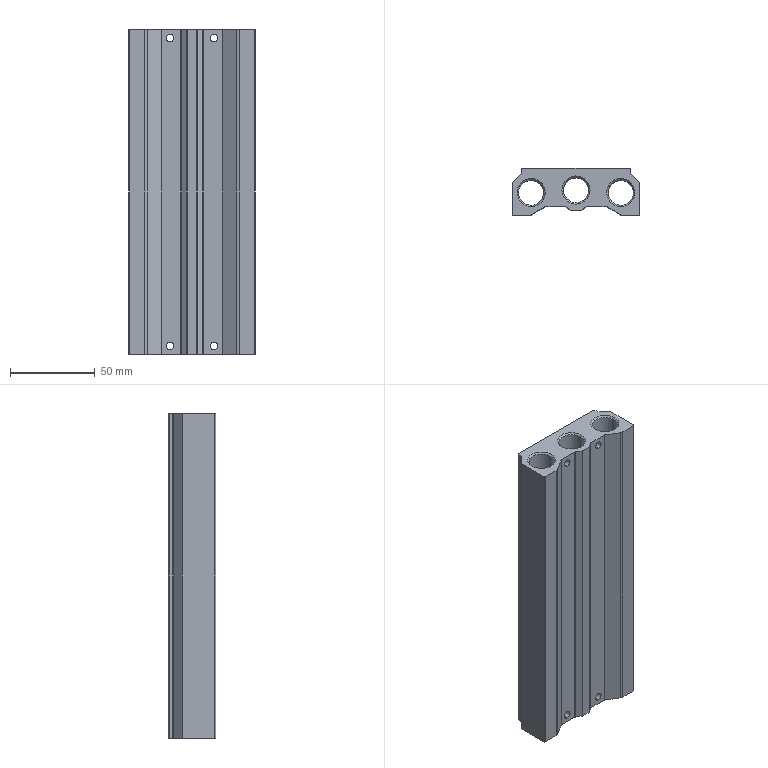Part | SolidWorks | features BaseBody 1 | 1 solid | 178 faces | box 75 x 28 x 192 mm | volume 234020 mm3 | cylinder 88 | cone 60 | plane 30 | commonest cylinder face diameters 3.242 x24 8.5 x24 1 x12 13 x12 4.5 x8 14.95 x6